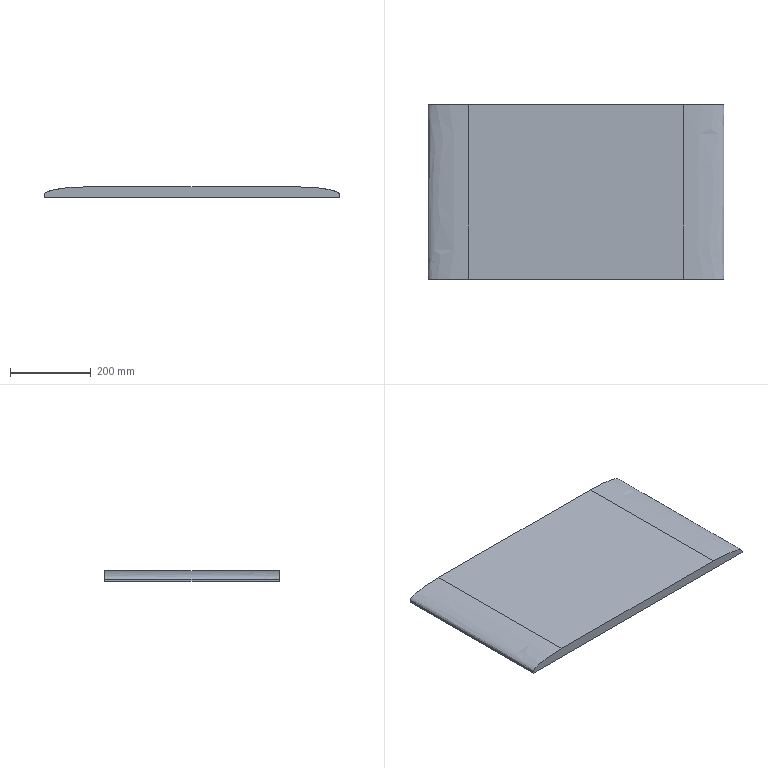Part | SolidWorks | features Fillet 2, Extrusion 1 | 1 solid | 8 faces | box 730 x 430 x 25.029 mm | volume 7503443 mm3 | plane 6 | spline 2
STEP:
#1=CARTESIAN_POINT('',(-365.,-215.,5.029));
#2=VERTEX_POINT('',#1);
#3=CARTESIAN_POINT('',(-365.,-215.,0.));
#4=VERTEX_POINT('',#3);
#5=CARTESIAN_POINT('',(-365.,-215.,25.029));
#6=DIRECTION('',(0.,0.,-1.));
#7=VECTOR('',#6,1000.);
#8=LINE('',#5,#7);
#9=EDGE_CURVE('',#2,#4,#8,.T.);
#10=ORIENTED_EDGE('',*,*,#9,.F.);
#11=CARTESIAN_POINT('',(-365.,215.,5.029));
#12=VERTEX_POINT('',#11);
#13=CARTESIAN_POINT('',(-365.,-215.,5.029));
#14=CARTESIAN_POINT('',(-365.,-71.667,5.029));
#15=CARTESIAN_POINT('',(-365.,71.667,5.029));
#16=CARTESIAN_POINT('',(-365.,215.,5.029));
#17=B_SPLINE_CURVE_WITH_KNOTS('',3,(#13,#14,#15,#16),.UNSPECIFIED.,.F.,.F.,(4,4),(0.,1.),.UNSPECIFIED.);
#18=EDGE_CURVE('',#2,#12,#17,.T.);
#19=ORIENTED_EDGE('',*,*,#18,.T.);
#20=CARTESIAN_POINT('',(-365.,215.,0.));
#21=VERTEX_POINT('',#20);
#22=CARTESIAN_POINT('',(-365.,215.,25.029));
#23=DIRECTION('',(0.,0.,-1.));
#24=VECTOR('',#23,1000.);
#25=LINE('',#22,#24);
#26=EDGE_CURVE('',#12,#21,#25,.T.);
#27=ORIENTED_EDGE('',*,*,#26,.T.);
#28=CARTESIAN_POINT('',(-365.,-215.,0.));
#29=DIRECTION('',(0.,-1.,0.));
#30=VECTOR('',#29,1000.);
#31=LINE('',#28,#30);
#32=EDGE_CURVE('',#21,#4,#31,.T.);
#33=ORIENTED_EDGE('',*,*,#32,.T.);
#34=EDGE_LOOP('',(#10,#19,#27,#33));
#35=FACE_OUTER_BOUND('',#34,.T.);
#36=CARTESIAN_POINT('',(-365.,-215.,25.029));
#37=DIRECTION('',(1.,0.,0.));
#38=DIRECTION('',(0.,0.,-1.));
#39=AXIS2_PLACEMENT_3D('',#36,#37,#38);
#40=PLANE('',#39);
#41=ADVANCED_FACE('',(#35),#40,.F.);
#42=CARTESIAN_POINT('',(365.,-215.,5.029));
#43=VERTEX_POINT('',#42);
#44=CARTESIAN_POINT('',(365.,-215.,0.));
#45=VERTEX_POINT('',#44);
#46=CARTESIAN_POINT('',(365.,-215.,25.029));
#47=DIRECTION('',(0.,0.,-1.));
#48=VECTOR('',#47,1000.);
#49=LINE('',#46,#48);
#50=EDGE_CURVE('',#43,#45,#49,.T.);
#51=ORIENTED_EDGE('',*,*,#50,.F.);
#52=CARTESIAN_POINT('',(265.,-215.,25.029));
#53=VERTEX_POINT('',#52);
#54=CARTESIAN_POINT('',(365.,-215.,5.029));
#55=CARTESIAN_POINT('',(365.,-215.,5.932));
#56=CARTESIAN_POINT('',(364.55,-215.,7.274));
#57=CARTESIAN_POINT('',(363.236,-215.,8.819));
#58=CARTESIAN_POINT('',(362.382,-215.,9.586));
#59=CARTESIAN_POINT('',(361.905,-215.,9.968));
#60=CARTESIAN_POINT('',(361.655,-215.,10.159));
#61=CARTESIAN_POINT('',(361.527,-215.,10.254));
#62=CARTESIAN_POINT('',(361.462,-215.,10.302));
#63=CARTESIAN_POINT('',(361.429,-215.,10.325));
#64=CARTESIAN_POINT('',(361.415,-215.,10.336));
#65=CARTESIAN_POINT('',(361.406,-215.,10.342));
#66=CARTESIAN_POINT('',(361.399,-215.,10.347));
#67=CARTESIAN_POINT('',(360.651,-215.,10.889));
#68=CARTESIAN_POINT('',(359.369,-215.,11.687));
#69=CARTESIAN_POINT('',(357.583,-215.,12.596));
#70=CARTESIAN_POINT('',(356.618,-215.,13.046));
#71=CARTESIAN_POINT('',(356.118,-215.,13.269));
#72=CARTESIAN_POINT('',(355.863,-215.,13.381));
#73=CARTESIAN_POINT('',(355.734,-215.,13.436));
#74=CARTESIAN_POINT('',(355.67,-215.,13.464));
#75=CARTESIAN_POINT('',(355.637,-215.,13.478));
#76=CARTESIAN_POINT('',(355.624,-215.,13.484));
#77=CARTESIAN_POINT('',(355.614,-215.,13.488));
#78=CARTESIAN_POINT('',(355.608,-215.,13.491));
#79=CARTESIAN_POINT('',(353.919,-215.,14.214));
#80=CARTESIAN_POINT('',(351.09,-215.,15.259));
#81=CARTESIAN_POINT('',(347.261,-215.,16.413));
#82=CARTESIAN_POINT('',(345.214,-215.,16.974));
#83=CARTESIAN_POINT('',(344.158,-215.,17.251));
#84=CARTESIAN_POINT('',(343.622,-215.,17.388));
#85=CARTESIAN_POINT('',(343.352,-215.,17.456));
#86=CARTESIAN_POINT('',(343.216,-215.,17.49));
#87=CARTESIAN_POINT('',(343.148,-215.,17.507));
#88=CARTESIAN_POINT('',(343.114,-215.,17.516));
#89=CARTESIAN_POINT('',(343.099,-215.,17.519));
#90=CARTESIAN_POINT('',(343.09,-215.,17.522));
#91=CARTESIAN_POINT('',(343.084,-215.,17.523));
#92=CARTESIAN_POINT('',(339.45,-215.,18.432));
#93=CARTESIAN_POINT('',(333.509,-215.,19.68));
#94=CARTESIAN_POINT('',(325.712,-215.,20.941));
#95=CARTESIAN_POINT('',(321.596,-215.,21.522));
#96=CARTESIAN_POINT('',(319.484,-215.,21.801));
#97=CARTESIAN_POINT('',(318.414,-215.,21.937));
#98=CARTESIAN_POINT('',(317.876,-215.,22.004));
#99=CARTESIAN_POINT('',(317.606,-215.,22.038));
#100=CARTESIAN_POINT('',(317.471,-215.,22.054));
#101=CARTESIAN_POINT('',(317.403,-215.,22.063));
#102=CARTESIAN_POINT('',(317.374,-215.,22.066));
#103=CARTESIAN_POINT('',(317.355,-215.,22.068));
#104=CARTESIAN_POINT('',(317.343,-215.,22.07));
#105=CARTESIAN_POINT('',(313.254,-215.,22.572));
#106=CARTESIAN_POINT('',(306.928,-215.,23.231));
#107=CARTESIAN_POINT('',(299.192,-215.,23.834));
#108=CARTESIAN_POINT('',(295.236,-215.,24.095));
#109=CARTESIAN_POINT('',(293.235,-215.,24.215));
#110=CARTESIAN_POINT('',(292.229,-215.,24.273));
#111=CARTESIAN_POINT('',(291.725,-215.,24.301));
#112=CARTESIAN_POINT('',(291.473,-215.,24.315));
#113=CARTESIAN_POINT('',(291.346,-215.,24.322));
#114=CARTESIAN_POINT('',(291.292,-215.,24.325));
#115=CARTESIAN_POINT('',(291.256,-215.,24.327));
#116=CARTESIAN_POINT('',(291.237,-215.,24.328));
#117=CARTESIAN_POINT('',(282.636,-215.,24.795));
#118=CARTESIAN_POINT('',(273.896,-215.,25.029));
#119=CARTESIAN_POINT('',(265.,-215.,25.029));
#120=B_SPLINE_CURVE_WITH_KNOTS('',3,(#54,#55,#56,#57,#58,#59,#60,#61,#62,#63,#64,#65,#66,#67,#68,#69,#70,#71,#72,#73,#74,#75,#76,#77,#78,#79,#80,#81,#82,#83,#84,#85,#86,#87,#88,#89,#90,#91,#92,#93,#94,#95,#96,#97,#98,#99,#100,#101,#102,#103,#104,#105,#106,#107,#108,#109,#110,#111,#112,#113,#114,#115,#116,#117,#118,#119),.UNSPECIFIED.,.F.,.F.,(4,1,1,1,1,1,1,1,1,2,2,1,1,1,1,1,1,1,1,2,2,1,1,1,1,1,1,1,1,1,2,2,1,1,1,1,1,1,1,1,1,2,2,1,1,1,1,1,1,1,1,2,2,4),(0.,0.03125,0.04687,0.05469,0.05859,0.06055,0.06152,0.06201,0.06226,0.06238,0.0625,0.09375,0.1094,0.1172,0.1211,0.123,0.124,0.1245,0.1248,0.1249,0.125,0.1875,0.2187,0.2344,0.2422,0.2461,0.248,0.249,0.2495,0.2498,0.2499,0.25,0.375,0.4375,0.4688,0.4844,0.4922,0.4961,0.498,0.499,0.4995,0.4998,0.5,0.625,0.6875,0.7188,0.7344,0.7422,0.7461,0.748,0.749,0.7495,0.75,1.),.UNSPECIFIED.);
#121=EDGE_CURVE('',#43,#53,#120,.T.);
#122=ORIENTED_EDGE('',*,*,#121,.T.);
#123=CARTESIAN_POINT('',(-265.,-215.,25.029));
#124=VERTEX_POINT('',#123);
#125=CARTESIAN_POINT('',(365.,-215.,25.029));
#126=DIRECTION('',(1.,0.,0.));
#127=VECTOR('',#126,1000.);
#128=LINE('',#125,#127);
#129=EDGE_CURVE('',#124,#53,#128,.T.);
#130=ORIENTED_EDGE('',*,*,#129,.F.);
#131=CARTESIAN_POINT('',(-265.,-215.,25.029));
#132=CARTESIAN_POINT('',(-269.45,-215.,25.029));
#133=CARTESIAN_POINT('',(-276.067,-215.,24.941));
#134=CARTESIAN_POINT('',(-283.685,-215.,24.686));
#135=CARTESIAN_POINT('',(-287.468,-215.,24.52));
#136=CARTESIAN_POINT('',(-289.353,-215.,24.427));
#137=CARTESIAN_POINT('',(-290.294,-215.,24.378));
#138=CARTESIAN_POINT('',(-290.764,-215.,24.353));
#139=CARTESIAN_POINT('',(-290.999,-215.,24.341));
#140=CARTESIAN_POINT('',(-291.116,-215.,24.334));
#141=CARTESIAN_POINT('',(-291.167,-215.,24.332));
#142=CARTESIAN_POINT('',(-291.2,-215.,24.33));
#143=CARTESIAN_POINT('',(-291.216,-215.,24.329));
#144=CARTESIAN_POINT('',(-295.864,-215.,24.076));
#145=CARTESIAN_POINT('',(-302.605,-215.,23.605));
#146=CARTESIAN_POINT('',(-310.113,-215.,22.89));
#147=CARTESIAN_POINT('',(-313.779,-215.,22.491));
#148=CARTESIAN_POINT('',(-315.589,-215.,22.281));
#149=CARTESIAN_POINT('',(-316.489,-215.,22.174));
#150=CARTESIAN_POINT('',(-316.937,-215.,22.12));
#151=CARTESIAN_POINT('',(-317.161,-215.,22.092));
#152=CARTESIAN_POINT('',(-317.273,-215.,22.079));
#153=CARTESIAN_POINT('',(-317.329,-215.,22.072));
#154=CARTESIAN_POINT('',(-317.353,-215.,22.069));
#155=CARTESIAN_POINT('',(-317.369,-215.,22.067));
#156=CARTESIAN_POINT('',(-317.375,-215.,22.066));
#157=CARTESIAN_POINT('',(-322.359,-215.,21.453));
#158=CARTESIAN_POINT('',(-329.32,-215.,20.422));
#159=CARTESIAN_POINT('',(-336.565,-215.,19.021));
#160=CARTESIAN_POINT('',(-339.968,-215.,18.271));
#161=CARTESIAN_POINT('',(-341.614,-215.,17.884));
#162=CARTESIAN_POINT('',(-342.424,-215.,17.687));
#163=CARTESIAN_POINT('',(-342.825,-215.,17.588));
#164=CARTESIAN_POINT('',(-343.025,-215.,17.538));
#165=CARTESIAN_POINT('',(-343.125,-215.,17.513));
#166=CARTESIAN_POINT('',(-343.175,-215.,17.5));
#167=CARTESIAN_POINT('',(-343.2,-215.,17.494));
#168=CARTESIAN_POINT('',(-343.21,-215.,17.492));
#169=CARTESIAN_POINT('',(-343.217,-215.,17.49));
#170=CARTESIAN_POINT('',(-343.22,-215.,17.489));
#171=CARTESIAN_POINT('',(-345.709,-215.,16.864));
#172=CARTESIAN_POINT('',(-349.134,-215.,15.891));
#173=CARTESIAN_POINT('',(-352.601,-215.,14.69));
#174=CARTESIAN_POINT('',(-354.202,-215.,14.073));
#175=CARTESIAN_POINT('',(-354.969,-215.,13.76));
#176=CARTESIAN_POINT('',(-355.345,-215.,13.603));
#177=CARTESIAN_POINT('',(-355.531,-215.,13.524));
#178=CARTESIAN_POINT('',(-355.623,-215.,13.484));
#179=CARTESIAN_POINT('',(-355.669,-215.,13.465));
#180=CARTESIAN_POINT('',(-355.692,-215.,13.455));
#181=CARTESIAN_POINT('',(-355.702,-215.,13.45));
#182=CARTESIAN_POINT('',(-355.708,-215.,13.448));
#183=CARTESIAN_POINT('',(-355.71,-215.,13.447));
#184=CARTESIAN_POINT('',(-356.892,-215.,12.937));
#185=CARTESIAN_POINT('',(-358.493,-215.,12.164));
#186=CARTESIAN_POINT('',(-360.072,-215.,11.241));
#187=CARTESIAN_POINT('',(-360.79,-215.,10.774));
#188=CARTESIAN_POINT('',(-361.131,-215.,10.539));
#189=CARTESIAN_POINT('',(-361.297,-215.,10.421));
#190=CARTESIAN_POINT('',(-361.379,-215.,10.362));
#191=CARTESIAN_POINT('',(-361.419,-215.,10.333));
#192=CARTESIAN_POINT('',(-361.44,-215.,10.318));
#193=CARTESIAN_POINT('',(-361.448,-215.,10.312));
#194=CARTESIAN_POINT('',(-361.454,-215.,10.307));
#195=CARTESIAN_POINT('',(-361.455,-215.,10.306));
#196=CARTESIAN_POINT('',(-363.82,-215.,8.577));
#197=CARTESIAN_POINT('',(-365.,-215.,6.819));
#198=CARTESIAN_POINT('',(-365.,-215.,5.029));
#199=B_SPLINE_CURVE_WITH_KNOTS('',3,(#131,#132,#133,#134,#135,#136,#137,#138,#139,#140,#141,#142,#143,#144,#145,#146,#147,#148,#149,#150,#151,#152,#153,#154,#155,#156,#157,#158,#159,#160,#161,#162,#163,#164,#165,#166,#167,#168,#169,#170,#171,#172,#173,#174,#175,#176,#177,#178,#179,#180,#181,#182,#183,#184,#185,#186,#187,#188,#189,#190,#191,#192,#193,#194,#195,#196,#197,#198),.UNSPECIFIED.,.F.,.F.,(4,1,1,1,1,1,1,1,1,2,2,1,1,1,1,1,1,1,1,1,2,2,1,1,1,1,1,1,1,1,1,1,2,2,1,1,1,1,1,1,1,1,1,2,2,1,1,1,1,1,1,1,1,2,2,4),(0.,0.125,0.1875,0.2188,0.2344,0.2422,0.2461,0.248,0.249,0.2495,0.25,0.375,0.4375,0.4688,0.4844,0.4922,0.4961,0.498,0.499,0.4995,0.4998,0.5,0.625,0.6875,0.7187,0.7344,0.7422,0.7461,0.748,0.749,0.7495,0.7498,0.7499,0.75,0.8125,0.8438,0.8594,0.8672,0.8711,0.873,0.874,0.8745,0.8748,0.8749,0.875,0.9063,0.9219,0.9297,0.9336,0.9355,0.9365,0.937,0.9373,0.9374,0.9375,1.),.UNSPECIFIED.);
#200=EDGE_CURVE('',#124,#2,#199,.T.);
#201=ORIENTED_EDGE('',*,*,#200,.T.);
#202=ORIENTED_EDGE('',*,*,#9,.T.);
#203=CARTESIAN_POINT('',(365.,-215.,0.));
#204=DIRECTION('',(1.,0.,0.));
#205=VECTOR('',#204,1000.);
#206=LINE('',#203,#205);
#207=EDGE_CURVE('',#4,#45,#206,.T.);
#208=ORIENTED_EDGE('',*,*,#207,.T.);
#209=EDGE_LOOP('',(#51,#122,#130,#201,#202,#208));
#210=FACE_OUTER_BOUND('',#209,.T.);
#211=CARTESIAN_POINT('',(365.,-215.,25.029));
#212=DIRECTION('',(0.,1.,0.));
#213=DIRECTION('',(-1.,0.,0.));
#214=AXIS2_PLACEMENT_3D('',#211,#212,#213);
#215=PLANE('',#214);
#216=ADVANCED_FACE('',(#210),#215,.F.);
#217=CARTESIAN_POINT('',(365.,215.,5.029));
#218=VERTEX_POINT('',#217);
#219=CARTESIAN_POINT('',(365.,215.,0.));
#220=VERTEX_POINT('',#219);
#221=CARTESIAN_POINT('',(365.,215.,25.029));
#222=DIRECTION('',(0.,0.,-1.));
#223=VECTOR('',#222,1000.);
#224=LINE('',#221,#223);
#225=EDGE_CURVE('',#218,#220,#224,.T.);
#226=ORIENTED_EDGE('',*,*,#225,.F.);
#227=CARTESIAN_POINT('',(365.,215.,5.029));
#228=CARTESIAN_POINT('',(365.,71.667,5.029));
#229=CARTESIAN_POINT('',(365.,-71.667,5.029));
#230=CARTESIAN_POINT('',(365.,-215.,5.029));
#231=B_SPLINE_CURVE_WITH_KNOTS('',3,(#227,#228,#229,#230),.UNSPECIFIED.,.F.,.F.,(4,4),(0.,1.),.UNSPECIFIED.);
#232=EDGE_CURVE('',#218,#43,#231,.T.);
#233=ORIENTED_EDGE('',*,*,#232,.T.);
#234=ORIENTED_EDGE('',*,*,#50,.T.);
#235=CARTESIAN_POINT('',(365.,-215.,0.));
#236=DIRECTION('',(0.,1.,0.));
#237=VECTOR('',#236,1000.);
#238=LINE('',#235,#237);
#239=EDGE_CURVE('',#45,#220,#238,.T.);
#240=ORIENTED_EDGE('',*,*,#239,.T.);
#241=EDGE_LOOP('',(#226,#233,#234,#240));
#242=FACE_OUTER_BOUND('',#241,.T.);
#243=CARTESIAN_POINT('',(365.,-215.,25.029));
#244=DIRECTION('',(-1.,0.,0.));
#245=DIRECTION('',(0.,0.,1.));
#246=AXIS2_PLACEMENT_3D('',#243,#244,#245);
#247=PLANE('',#246);
#248=ADVANCED_FACE('',(#242),#247,.F.);
#249=CARTESIAN_POINT('',(265.,215.,25.029));
#250=VERTEX_POINT('',#249);
#251=CARTESIAN_POINT('',(-265.,215.,25.029));
#252=VERTEX_POINT('',#251);
#253=CARTESIAN_POINT('',(365.,215.,25.029));
#254=DIRECTION('',(-1.,0.,0.));
#255=VECTOR('',#254,1000.);
#256=LINE('',#253,#255);
#257=EDGE_CURVE('',#250,#252,#256,.T.);
#258=ORIENTED_EDGE('',*,*,#257,.F.);
#259=CARTESIAN_POINT('',(265.,215.,25.029));
#260=CARTESIAN_POINT('',(269.45,215.,25.029));
#261=CARTESIAN_POINT('',(276.067,215.,24.941));
#262=CARTESIAN_POINT('',(283.685,215.,24.686));
#263=CARTESIAN_POINT('',(287.468,215.,24.52));
#264=CARTESIAN_POINT('',(289.353,215.,24.427));
#265=CARTESIAN_POINT('',(290.294,215.,24.378));
#266=CARTESIAN_POINT('',(290.764,215.,24.353));
#267=CARTESIAN_POINT('',(290.999,215.,24.341));
#268=CARTESIAN_POINT('',(291.116,215.,24.334));
#269=CARTESIAN_POINT('',(291.167,215.,24.332));
#270=CARTESIAN_POINT('',(291.2,215.,24.33));
#271=CARTESIAN_POINT('',(291.216,215.,24.329));
#272=CARTESIAN_POINT('',(295.864,215.,24.076));
#273=CARTESIAN_POINT('',(302.605,215.,23.605));
#274=CARTESIAN_POINT('',(310.113,215.,22.89));
#275=CARTESIAN_POINT('',(313.779,215.,22.491));
#276=CARTESIAN_POINT('',(315.589,215.,22.281));
#277=CARTESIAN_POINT('',(316.489,215.,22.174));
#278=CARTESIAN_POINT('',(316.937,215.,22.12));
#279=CARTESIAN_POINT('',(317.161,215.,22.092));
#280=CARTESIAN_POINT('',(317.273,215.,22.079));
#281=CARTESIAN_POINT('',(317.329,215.,22.072));
#282=CARTESIAN_POINT('',(317.353,215.,22.069));
#283=CARTESIAN_POINT('',(317.369,215.,22.067));
#284=CARTESIAN_POINT('',(317.375,215.,22.066));
#285=CARTESIAN_POINT('',(322.359,215.,21.453));
#286=CARTESIAN_POINT('',(329.32,215.,20.422));
#287=CARTESIAN_POINT('',(336.565,215.,19.021));
#288=CARTESIAN_POINT('',(339.968,215.,18.271));
#289=CARTESIAN_POINT('',(341.614,215.,17.884));
#290=CARTESIAN_POINT('',(342.424,215.,17.687));
#291=CARTESIAN_POINT('',(342.825,215.,17.588));
#292=CARTESIAN_POINT('',(343.025,215.,17.538));
#293=CARTESIAN_POINT('',(343.125,215.,17.513));
#294=CARTESIAN_POINT('',(343.175,215.,17.5));
#295=CARTESIAN_POINT('',(343.2,215.,17.494));
#296=CARTESIAN_POINT('',(343.21,215.,17.492));
#297=CARTESIAN_POINT('',(343.217,215.,17.49));
#298=CARTESIAN_POINT('',(343.22,215.,17.489));
#299=CARTESIAN_POINT('',(345.709,215.,16.864));
#300=CARTESIAN_POINT('',(349.134,215.,15.891));
#301=CARTESIAN_POINT('',(352.601,215.,14.69));
#302=CARTESIAN_POINT('',(354.202,215.,14.073));
#303=CARTESIAN_POINT('',(354.969,215.,13.76));
#304=CARTESIAN_POINT('',(355.345,215.,13.603));
#305=CARTESIAN_POINT('',(355.531,215.,13.524));
#306=CARTESIAN_POINT('',(355.623,215.,13.484));
#307=CARTESIAN_POINT('',(355.669,215.,13.465));
#308=CARTESIAN_POINT('',(355.692,215.,13.455));
#309=CARTESIAN_POINT('',(355.702,215.,13.45));
#310=CARTESIAN_POINT('',(355.708,215.,13.448));
#311=CARTESIAN_POINT('',(355.71,215.,13.447));
#312=CARTESIAN_POINT('',(356.892,215.,12.937));
#313=CARTESIAN_POINT('',(358.493,215.,12.164));
#314=CARTESIAN_POINT('',(360.072,215.,11.241));
#315=CARTESIAN_POINT('',(360.79,215.,10.774));
#316=CARTESIAN_POINT('',(361.131,215.,10.539));
#317=CARTESIAN_POINT('',(361.297,215.,10.421));
#318=CARTESIAN_POINT('',(361.379,215.,10.362));
#319=CARTESIAN_POINT('',(361.419,215.,10.333));
#320=CARTESIAN_POINT('',(361.44,215.,10.318));
#321=CARTESIAN_POINT('',(361.448,215.,10.312));
#322=CARTESIAN_POINT('',(361.454,215.,10.307));
#323=CARTESIAN_POINT('',(361.455,215.,10.306));
#324=CARTESIAN_POINT('',(363.82,215.,8.577));
#325=CARTESIAN_POINT('',(365.,215.,6.819));
#326=CARTESIAN_POINT('',(365.,215.,5.029));
#327=B_SPLINE_CURVE_WITH_KNOTS('',3,(#259,#260,#261,#262,#263,#264,#265,#266,#267,#268,#269,#270,#271,#272,#273,#274,#275,#276,#277,#278,#279,#280,#281,#282,#283,#284,#285,#286,#287,#288,#289,#290,#291,#292,#293,#294,#295,#296,#297,#298,#299,#300,#301,#302,#303,#304,#305,#306,#307,#308,#309,#310,#311,#312,#313,#314,#315,#316,#317,#318,#319,#320,#321,#322,#323,#324,#325,#326),.UNSPECIFIED.,.F.,.F.,(4,1,1,1,1,1,1,1,1,2,2,1,1,1,1,1,1,1,1,1,2,2,1,1,1,1,1,1,1,1,1,1,2,2,1,1,1,1,1,1,1,1,1,2,2,1,1,1,1,1,1,1,1,2,2,4),(0.,0.125,0.1875,0.2187,0.2344,0.2422,0.2461,0.248,0.249,0.2495,0.25,0.375,0.4375,0.4687,0.4844,0.4922,0.4961,0.498,0.499,0.4995,0.4998,0.5,0.625,0.6875,0.7187,0.7344,0.7422,0.7461,0.748,0.749,0.7495,0.7498,0.7499,0.75,0.8125,0.8437,0.8594,0.8672,0.8711,0.873,0.874,0.8745,0.8748,0.8749,0.875,0.9062,0.9219,0.9297,0.9336,0.9355,0.9365,0.937,0.9373,0.9374,0.9375,1.),.UNSPECIFIED.);
#328=EDGE_CURVE('',#250,#218,#327,.T.);
#329=ORIENTED_EDGE('',*,*,#328,.T.);
#330=ORIENTED_EDGE('',*,*,#225,.T.);
#331=CARTESIAN_POINT('',(365.,215.,0.));
#332=DIRECTION('',(-1.,0.,0.));
#333=VECTOR('',#332,1000.);
#334=LINE('',#331,#333);
#335=EDGE_CURVE('',#220,#21,#334,.T.);
#336=ORIENTED_EDGE('',*,*,#335,.T.);
#337=ORIENTED_EDGE('',*,*,#26,.F.);
#338=CARTESIAN_POINT('',(-365.,215.,5.029));
#339=CARTESIAN_POINT('',(-365.,215.,5.932));
#340=CARTESIAN_POINT('',(-364.55,215.,7.274));
#341=CARTESIAN_POINT('',(-363.236,215.,8.819));
#342=CARTESIAN_POINT('',(-362.382,215.,9.586));
#343=CARTESIAN_POINT('',(-361.905,215.,9.968));
#344=CARTESIAN_POINT('',(-361.655,215.,10.159));
#345=CARTESIAN_POINT('',(-361.527,215.,10.254));
#346=CARTESIAN_POINT('',(-361.462,215.,10.302));
#347=CARTESIAN_POINT('',(-361.429,215.,10.325));
#348=CARTESIAN_POINT('',(-361.415,215.,10.336));
#349=CARTESIAN_POINT('',(-361.406,215.,10.342));
#350=CARTESIAN_POINT('',(-361.399,215.,10.347));
#351=CARTESIAN_POINT('',(-360.651,215.,10.889));
#352=CARTESIAN_POINT('',(-359.369,215.,11.687));
#353=CARTESIAN_POINT('',(-357.583,215.,12.596));
#354=CARTESIAN_POINT('',(-356.618,215.,13.046));
#355=CARTESIAN_POINT('',(-356.118,215.,13.269));
#356=CARTESIAN_POINT('',(-355.863,215.,13.381));
#357=CARTESIAN_POINT('',(-355.734,215.,13.436));
#358=CARTESIAN_POINT('',(-355.67,215.,13.464));
#359=CARTESIAN_POINT('',(-355.637,215.,13.478));
#360=CARTESIAN_POINT('',(-355.624,215.,13.484));
#361=CARTESIAN_POINT('',(-355.614,215.,13.488));
#362=CARTESIAN_POINT('',(-355.608,215.,13.491));
#363=CARTESIAN_POINT('',(-353.919,215.,14.214));
#364=CARTESIAN_POINT('',(-351.09,215.,15.259));
#365=CARTESIAN_POINT('',(-347.261,215.,16.413));
#366=CARTESIAN_POINT('',(-345.214,215.,16.974));
#367=CARTESIAN_POINT('',(-344.158,215.,17.251));
#368=CARTESIAN_POINT('',(-343.622,215.,17.388));
#369=CARTESIAN_POINT('',(-343.352,215.,17.456));
#370=CARTESIAN_POINT('',(-343.216,215.,17.49));
#371=CARTESIAN_POINT('',(-343.148,215.,17.507));
#372=CARTESIAN_POINT('',(-343.114,215.,17.516));
#373=CARTESIAN_POINT('',(-343.099,215.,17.519));
#374=CARTESIAN_POINT('',(-343.09,215.,17.522));
#375=CARTESIAN_POINT('',(-343.084,215.,17.523));
#376=CARTESIAN_POINT('',(-339.45,215.,18.432));
#377=CARTESIAN_POINT('',(-333.509,215.,19.68));
#378=CARTESIAN_POINT('',(-325.712,215.,20.941));
#379=CARTESIAN_POINT('',(-321.596,215.,21.522));
#380=CARTESIAN_POINT('',(-319.484,215.,21.801));
#381=CARTESIAN_POINT('',(-318.414,215.,21.937));
#382=CARTESIAN_POINT('',(-317.876,215.,22.004));
#383=CARTESIAN_POINT('',(-317.606,215.,22.038));
#384=CARTESIAN_POINT('',(-317.471,215.,22.054));
#385=CARTESIAN_POINT('',(-317.403,215.,22.063));
#386=CARTESIAN_POINT('',(-317.374,215.,22.066));
#387=CARTESIAN_POINT('',(-317.355,215.,22.068));
#388=CARTESIAN_POINT('',(-317.343,215.,22.07));
#389=CARTESIAN_POINT('',(-313.254,215.,22.572));
#390=CARTESIAN_POINT('',(-306.928,215.,23.231));
#391=CARTESIAN_POINT('',(-299.192,215.,23.834));
#392=CARTESIAN_POINT('',(-295.236,215.,24.095));
#393=CARTESIAN_POINT('',(-293.235,215.,24.215));
#394=CARTESIAN_POINT('',(-292.229,215.,24.273));
#395=CARTESIAN_POINT('',(-291.725,215.,24.301));
#396=CARTESIAN_POINT('',(-291.473,215.,24.315));
#397=CARTESIAN_POINT('',(-291.346,215.,24.322));
#398=CARTESIAN_POINT('',(-291.292,215.,24.325));
#399=CARTESIAN_POINT('',(-291.256,215.,24.327));
#400=CARTESIAN_POINT('',(-291.237,215.,24.328));
#401=CARTESIAN_POINT('',(-282.636,215.,24.795));
#402=CARTESIAN_POINT('',(-273.896,215.,25.029));
#403=CARTESIAN_POINT('',(-265.,215.,25.029));
#404=B_SPLINE_CURVE_WITH_KNOTS('',3,(#338,#339,#340,#341,#342,#343,#344,#345,#346,#347,#348,#349,#350,#351,#352,#353,#354,#355,#356,#357,#358,#359,#360,#361,#362,#363,#364,#365,#366,#367,#368,#369,#370,#371,#372,#373,#374,#375,#376,#377,#378,#379,#380,#381,#382,#383,#384,#385,#386,#387,#388,#389,#390,#391,#392,#393,#394,#395,#396,#397,#398,#399,#400,#401,#402,#403),.UNSPECIFIED.,.F.,.F.,(4,1,1,1,1,1,1,1,1,2,2,1,1,1,1,1,1,1,1,2,2,1,1,1,1,1,1,1,1,1,2,2,1,1,1,1,1,1,1,1,1,2,2,1,1,1,1,1,1,1,1,2,2,4),(0.,0.03125,0.04688,0.05469,0.05859,0.06055,0.06152,0.06201,0.06226,0.06238,0.0625,0.09375,0.1094,0.1172,0.1211,0.123,0.124,0.1245,0.1248,0.1249,0.125,0.1875,0.2187,0.2344,0.2422,0.2461,0.248,0.249,0.2495,0.2498,0.2499,0.25,0.375,0.4375,0.4687,0.4844,0.4922,0.4961,0.498,0.499,0.4995,0.4998,0.5,0.625,0.6875,0.7187,0.7344,0.7422,0.7461,0.748,0.749,0.7495,0.75,1.),.UNSPECIFIED.);
#405=EDGE_CURVE('',#12,#252,#404,.T.);
#406=ORIENTED_EDGE('',*,*,#405,.T.);
#407=EDGE_LOOP('',(#258,#329,#330,#336,#337,#406));
#408=FACE_OUTER_BOUND('',#407,.T.);
#409=CARTESIAN_POINT('',(365.,215.,25.029));
#410=DIRECTION('',(0.,-1.,0.));
#411=DIRECTION('',(1.,0.,0.));
#412=AXIS2_PLACEMENT_3D('',#409,#410,#411);
#413=PLANE('',#412);
#414=ADVANCED_FACE('',(#408),#413,.F.);
#415=ORIENTED_EDGE('',*,*,#129,.T.);
#416=CARTESIAN_POINT('',(265.,-215.,25.029));
#417=CARTESIAN_POINT('',(265.,-71.667,25.029));
#418=CARTESIAN_POINT('',(265.,71.667,25.029));
#419=CARTESIAN_POINT('',(265.,215.,25.029));
#420=B_SPLINE_CURVE_WITH_KNOTS('',3,(#416,#417,#418,#419),.UNSPECIFIED.,.F.,.F.,(4,4),(0.,1.),.UNSPECIFIED.);
#421=EDGE_CURVE('',#53,#250,#420,.T.);
#422=ORIENTED_EDGE('',*,*,#421,.T.);
#423=ORIENTED_EDGE('',*,*,#257,.T.);
#424=CARTESIAN_POINT('',(-265.,215.,25.029));
#425=CARTESIAN_POINT('',(-265.,71.667,25.029));
#426=CARTESIAN_POINT('',(-265.,-71.667,25.029));
#427=CARTESIAN_POINT('',(-265.,-215.,25.029));
#428=B_SPLINE_CURVE_WITH_KNOTS('',3,(#424,#425,#426,#427),.UNSPECIFIED.,.F.,.F.,(4,4),(0.,1.),.UNSPECIFIED.);
#429=EDGE_CURVE('',#252,#124,#428,.T.);
#430=ORIENTED_EDGE('',*,*,#429,.T.);
#431=EDGE_LOOP('',(#415,#422,#423,#430));
#432=FACE_OUTER_BOUND('',#431,.T.);
#433=CARTESIAN_POINT('',(0.,0.,25.029));
#434=DIRECTION('',(0.,0.,1.));
#435=DIRECTION('',(1.,0.,0.));
#436=AXIS2_PLACEMENT_3D('',#433,#434,#435);
#437=PLANE('',#436);
#438=ADVANCED_FACE('',(#432),#437,.T.);
#439=ORIENTED_EDGE('',*,*,#32,.F.);
#440=ORIENTED_EDGE('',*,*,#335,.F.);
#441=ORIENTED_EDGE('',*,*,#239,.F.);
#442=ORIENTED_EDGE('',*,*,#207,.F.);
#443=EDGE_LOOP('',(#439,#440,#441,#442));
#444=FACE_OUTER_BOUND('',#443,.T.);
#445=CARTESIAN_POINT('',(0.,0.,0.));
#446=DIRECTION('',(0.,0.,1.));
#447=DIRECTION('',(1.,0.,0.));
#448=AXIS2_PLACEMENT_3D('',#445,#446,#447);
#449=PLANE('',#448);
#450=ADVANCED_FACE('',(#444),#449,.F.);
#451=ORIENTED_EDGE('',*,*,#405,.F.);
#452=ORIENTED_EDGE('',*,*,#18,.F.);
#453=ORIENTED_EDGE('',*,*,#200,.F.);
#454=ORIENTED_EDGE('',*,*,#429,.F.);
#455=EDGE_LOOP('',(#451,#452,#453,#454));
#456=FACE_OUTER_BOUND('',#455,.T.);
#457=CARTESIAN_POINT('',(-365.,-236.5,5.029));
#458=CARTESIAN_POINT('',(-365.,-78.833,5.029));
#459=CARTESIAN_POINT('',(-365.,78.833,5.029));
#460=CARTESIAN_POINT('',(-365.,236.5,5.029));
#461=CARTESIAN_POINT('',(-365.,-236.5,25.029));
#462=CARTESIAN_POINT('',(-365.,-78.833,25.029));
#463=CARTESIAN_POINT('',(-365.,78.833,25.029));
#464=CARTESIAN_POINT('',(-365.,236.5,25.029));
#465=CARTESIAN_POINT('',(-265.,-236.5,25.029));
#466=CARTESIAN_POINT('',(-265.,-78.833,25.029));
#467=CARTESIAN_POINT('',(-265.,78.833,25.029));
#468=CARTESIAN_POINT('',(-265.,236.5,25.029));
#469=(BOUNDED_SURFACE()B_SPLINE_SURFACE(2,3,((#457,#458,#459,#460),(#461,#462,#463,#464),(#465,#466,#467,#468)),.UNSPECIFIED.,.F.,.F.,.T.)B_SPLINE_SURFACE_WITH_KNOTS((3,3),(4,4),(0.,1.),(-0.2365,0.2365),.UNSPECIFIED.)GEOMETRIC_REPRESENTATION_ITEM()RATIONAL_B_SPLINE_SURFACE(((1.,1.,1.,1.),(0.7071,0.7071,0.7071,0.7071),(1.,1.,1.,1.)))REPRESENTATION_ITEM('')SURFACE());
#470=ADVANCED_FACE('',(#456),#469,.T.);
#471=ORIENTED_EDGE('',*,*,#121,.F.);
#472=ORIENTED_EDGE('',*,*,#232,.F.);
#473=ORIENTED_EDGE('',*,*,#328,.F.);
#474=ORIENTED_EDGE('',*,*,#421,.F.);
#475=EDGE_LOOP('',(#471,#472,#473,#474));
#476=FACE_OUTER_BOUND('',#475,.T.);
#477=CARTESIAN_POINT('',(365.,236.5,5.029));
#478=CARTESIAN_POINT('',(365.,78.833,5.029));
#479=CARTESIAN_POINT('',(365.,-78.833,5.029));
#480=CARTESIAN_POINT('',(365.,-236.5,5.029));
#481=CARTESIAN_POINT('',(365.,236.5,25.029));
#482=CARTESIAN_POINT('',(365.,78.833,25.029));
#483=CARTESIAN_POINT('',(365.,-78.833,25.029));
#484=CARTESIAN_POINT('',(365.,-236.5,25.029));
#485=CARTESIAN_POINT('',(265.,236.5,25.029));
#486=CARTESIAN_POINT('',(265.,78.833,25.029));
#487=CARTESIAN_POINT('',(265.,-78.833,25.029));
#488=CARTESIAN_POINT('',(265.,-236.5,25.029));
#489=(BOUNDED_SURFACE()B_SPLINE_SURFACE(2,3,((#477,#478,#479,#480),(#481,#482,#483,#484),(#485,#486,#487,#488)),.UNSPECIFIED.,.F.,.F.,.T.)B_SPLINE_SURFACE_WITH_KNOTS((3,3),(4,4),(0.,1.),(-0.2365,0.2365),.UNSPECIFIED.)GEOMETRIC_REPRESENTATION_ITEM()RATIONAL_B_SPLINE_SURFACE(((1.,1.,1.,1.),(0.7071,0.7071,0.7071,0.7071),(1.,1.,1.,1.)))REPRESENTATION_ITEM('')SURFACE());
#490=ADVANCED_FACE('',(#476),#489,.T.);
#491=CLOSED_SHELL('',(#41,#216,#248,#414,#438,#450,#470,#490));
#492=MANIFOLD_SOLID_BREP('',#491);
#493=CARTESIAN_POINT('',(0.,0.,0.));
#494=DIRECTION('',(0.,0.,1.));
#495=DIRECTION('',(1.,0.,0.));
#496=AXIS2_PLACEMENT_3D('',#493,#494,#495);
#497=(LENGTH_UNIT()NAMED_UNIT(*)SI_UNIT(.MILLI.,.METRE.));
#498=UNCERTAINTY_MEASURE_WITH_UNIT(LENGTH_MEASURE(0.00001),#497,'','');
#499=(NAMED_UNIT(*)PLANE_ANGLE_UNIT()SI_UNIT($,.RADIAN.));
#500=(NAMED_UNIT(*)SI_UNIT($,.STERADIAN.)SOLID_ANGLE_UNIT());
#501=(GEOMETRIC_REPRESENTATION_CONTEXT(3)GLOBAL_UNCERTAINTY_ASSIGNED_CONTEXT((#498))GLOBAL_UNIT_ASSIGNED_CONTEXT((#497,#499,#500))REPRESENTATION_CONTEXT('',''));
#502=ADVANCED_BREP_SHAPE_REPRESENTATION('',(#492,#496),#501);